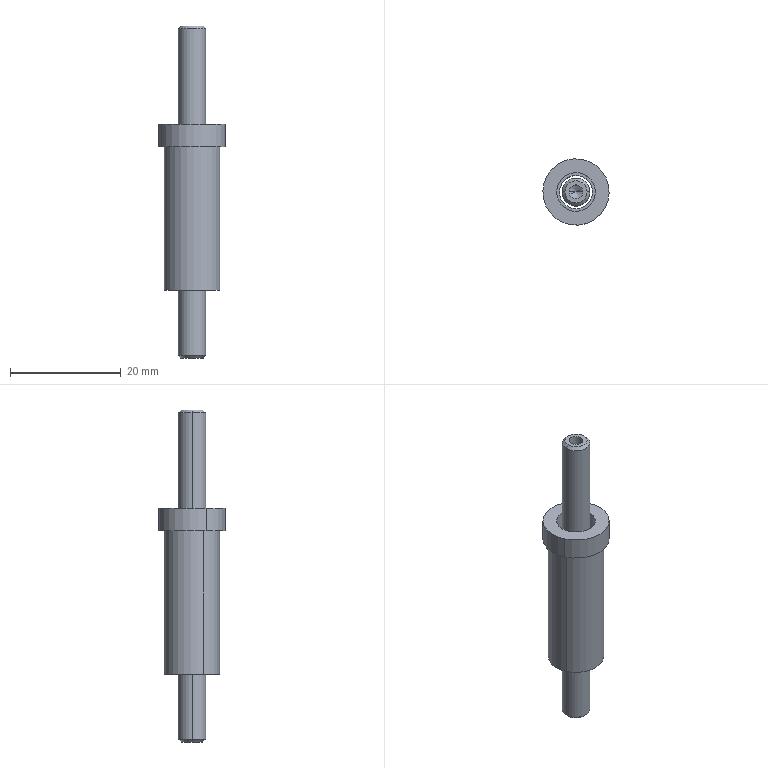Part | NX | features BREP 2 | 2 solids | 31 faces | box 12 x 12 x 60 mm | volume 2642 mm3 | cylinder 16 | cone 8 | plane 7 | commonest cylinder face diameters 2.5 x4 7 x4 5 x2 6 x2 10 x2 12 x2
STEP:
#1=CARTESIAN_POINT('',(-71.096,14.282,-29.5));
#2=VERTEX_POINT('',#1);
#3=CARTESIAN_POINT('',(-70.596,14.282,-30.));
#4=VERTEX_POINT('',#3);
#5=CARTESIAN_POINT('',(-71.096,14.282,-29.5));
#6=DIRECTION('',(-0.7071,0.,0.7071));
#7=VECTOR('',#6,1000.);
#8=LINE('',#5,#7);
#9=EDGE_CURVE('',#2,#4,#8,.F.);
#10=ORIENTED_EDGE('',*,*,#9,.T.);
#11=CARTESIAN_POINT('',(-66.596,14.282,-30.));
#12=VERTEX_POINT('',#11);
#13=CARTESIAN_POINT('',(-68.596,14.282,-30.));
#14=DIRECTION('',(0.,0.,-1.));
#15=DIRECTION('',(1.,0.,0.));
#16=AXIS2_PLACEMENT_3D('',#13,#14,#15);
#17=CIRCLE('',#16,2.);
#18=EDGE_CURVE('',#12,#4,#17,.T.);
#19=ORIENTED_EDGE('',*,*,#18,.F.);
#20=CARTESIAN_POINT('',(-66.096,14.282,-29.5));
#21=VERTEX_POINT('',#20);
#22=CARTESIAN_POINT('',(-66.096,14.282,-29.5));
#23=DIRECTION('',(0.7071,0.,0.7071));
#24=VECTOR('',#23,1000.);
#25=LINE('',#22,#24);
#26=EDGE_CURVE('',#21,#12,#25,.F.);
#27=ORIENTED_EDGE('',*,*,#26,.F.);
#28=CARTESIAN_POINT('',(-68.596,14.282,-29.5));
#29=DIRECTION('',(0.,0.,1.));
#30=DIRECTION('',(1.,0.,0.));
#31=AXIS2_PLACEMENT_3D('',#28,#29,#30);
#32=CIRCLE('',#31,2.5);
#33=EDGE_CURVE('',#2,#21,#32,.T.);
#34=ORIENTED_EDGE('',*,*,#33,.F.);
#35=EDGE_LOOP('',(#10,#19,#27,#34));
#36=FACE_BOUND('',#35,.T.);
#37=CARTESIAN_POINT('',(-68.596,14.282,-29.5));
#38=DIRECTION('',(0.,0.,1.));
#39=DIRECTION('',(1.,0.,0.));
#40=AXIS2_PLACEMENT_3D('',#37,#38,#39);
#41=CONICAL_SURFACE('',#40,2.5,0.7854);
#42=ADVANCED_FACE('',(#36),#41,.T.);
#43=CARTESIAN_POINT('',(-66.596,14.282,30.));
#44=VERTEX_POINT('',#43);
#45=CARTESIAN_POINT('',(-66.096,14.282,29.5));
#46=VERTEX_POINT('',#45);
#47=CARTESIAN_POINT('',(-66.596,14.282,30.));
#48=DIRECTION('',(0.7071,0.,-0.7071));
#49=VECTOR('',#48,1000.);
#50=LINE('',#47,#49);
#51=EDGE_CURVE('',#44,#46,#50,.T.);
#52=ORIENTED_EDGE('',*,*,#51,.F.);
#53=CARTESIAN_POINT('',(-70.596,14.282,30.));
#54=VERTEX_POINT('',#53);
#55=CARTESIAN_POINT('',(-68.596,14.282,30.));
#56=DIRECTION('',(0.,0.,1.));
#57=DIRECTION('',(1.,0.,0.));
#58=AXIS2_PLACEMENT_3D('',#55,#56,#57);
#59=CIRCLE('',#58,2.);
#60=EDGE_CURVE('',#54,#44,#59,.T.);
#61=ORIENTED_EDGE('',*,*,#60,.F.);
#62=CARTESIAN_POINT('',(-71.096,14.282,29.5));
#63=VERTEX_POINT('',#62);
#64=CARTESIAN_POINT('',(-70.596,14.282,30.));
#65=DIRECTION('',(-0.7071,0.,-0.7071));
#66=VECTOR('',#65,1000.);
#67=LINE('',#64,#66);
#68=EDGE_CURVE('',#54,#63,#67,.T.);
#69=ORIENTED_EDGE('',*,*,#68,.T.);
#70=CARTESIAN_POINT('',(-68.596,14.282,29.5));
#71=DIRECTION('',(0.,0.,-1.));
#72=DIRECTION('',(1.,0.,0.));
#73=AXIS2_PLACEMENT_3D('',#70,#71,#72);
#74=CIRCLE('',#73,2.5);
#75=EDGE_CURVE('',#46,#63,#74,.T.);
#76=ORIENTED_EDGE('',*,*,#75,.F.);
#77=EDGE_LOOP('',(#52,#61,#69,#76));
#78=FACE_BOUND('',#77,.T.);
#79=CARTESIAN_POINT('',(-68.596,14.282,30.));
#80=DIRECTION('',(0.,0.,-1.));
#81=DIRECTION('',(-1.,0.,0.));
#82=AXIS2_PLACEMENT_3D('',#79,#80,#81);
#83=CONICAL_SURFACE('',#82,2.,0.7854);
#84=ADVANCED_FACE('',(#78),#83,.T.);
#85=CARTESIAN_POINT('',(-69.846,14.282,30.));
#86=VERTEX_POINT('',#85);
#87=CARTESIAN_POINT('',(-69.846,14.282,22.5));
#88=VERTEX_POINT('',#87);
#89=CARTESIAN_POINT('',(-69.846,14.282,30.));
#90=DIRECTION('',(0.,0.,1.));
#91=VECTOR('',#90,1000.);
#92=LINE('',#89,#91);
#93=EDGE_CURVE('',#86,#88,#92,.F.);
#94=ORIENTED_EDGE('',*,*,#93,.T.);
#95=CARTESIAN_POINT('',(-67.346,14.282,22.5));
#96=VERTEX_POINT('',#95);
#97=CARTESIAN_POINT('',(-68.596,14.282,22.5));
#98=DIRECTION('',(0.,0.,1.));
#99=DIRECTION('',(1.,0.,0.));
#100=AXIS2_PLACEMENT_3D('',#97,#98,#99);
#101=CIRCLE('',#100,1.25);
#102=EDGE_CURVE('',#96,#88,#101,.T.);
#103=ORIENTED_EDGE('',*,*,#102,.F.);
#104=CARTESIAN_POINT('',(-67.346,14.282,30.));
#105=VERTEX_POINT('',#104);
#106=CARTESIAN_POINT('',(-67.346,14.282,30.));
#107=DIRECTION('',(0.,0.,1.));
#108=VECTOR('',#107,1000.);
#109=LINE('',#106,#108);
#110=EDGE_CURVE('',#105,#96,#109,.F.);
#111=ORIENTED_EDGE('',*,*,#110,.F.);
#112=CARTESIAN_POINT('',(-68.596,14.282,30.));
#113=DIRECTION('',(0.,0.,1.));
#114=DIRECTION('',(1.,0.,0.));
#115=AXIS2_PLACEMENT_3D('',#112,#113,#114);
#116=CIRCLE('',#115,1.25);
#117=EDGE_CURVE('',#105,#86,#116,.T.);
#118=ORIENTED_EDGE('',*,*,#117,.T.);
#119=EDGE_LOOP('',(#94,#103,#111,#118));
#120=FACE_BOUND('',#119,.T.);
#121=CARTESIAN_POINT('',(-68.596,14.282,30.));
#122=DIRECTION('',(0.,0.,1.));
#123=DIRECTION('',(1.,0.,0.));
#124=AXIS2_PLACEMENT_3D('',#121,#122,#123);
#125=CYLINDRICAL_SURFACE('',#124,1.25);
#126=ADVANCED_FACE('',(#120),#125,.F.);
#127=CARTESIAN_POINT('',(-68.596,14.282,21.749));
#128=VERTEX_POINT('',#127);
#129=CARTESIAN_POINT('',(-69.846,14.282,22.5));
#130=DIRECTION('',(-0.8572,0.,0.515));
#131=VECTOR('',#130,1000.);
#132=LINE('',#129,#131);
#133=EDGE_CURVE('',#128,#88,#132,.T.);
#134=ORIENTED_EDGE('',*,*,#133,.F.);
#135=CARTESIAN_POINT('',(-67.346,14.282,22.5));
#136=DIRECTION('',(0.8572,0.,0.515));
#137=VECTOR('',#136,1000.);
#138=LINE('',#135,#137);
#139=EDGE_CURVE('',#128,#96,#138,.T.);
#140=ORIENTED_EDGE('',*,*,#139,.T.);
#141=ORIENTED_EDGE('',*,*,#102,.T.);
#142=EDGE_LOOP('',(#134,#140,#141));
#143=FACE_BOUND('',#142,.T.);
#144=CARTESIAN_POINT('',(-68.596,14.282,22.5));
#145=DIRECTION('',(0.,0.,1.));
#146=DIRECTION('',(1.,0.,0.));
#147=AXIS2_PLACEMENT_3D('',#144,#145,#146);
#148=CONICAL_SURFACE('',#147,1.25,1.03);
#149=ADVANCED_FACE('',(#143),#148,.F.);
#150=CARTESIAN_POINT('',(-67.346,14.282,-22.5));
#151=VERTEX_POINT('',#150);
#152=CARTESIAN_POINT('',(-67.346,14.282,-30.));
#153=VERTEX_POINT('',#152);
#154=CARTESIAN_POINT('',(-67.346,14.282,-30.));
#155=DIRECTION('',(0.,0.,-1.));
#156=VECTOR('',#155,1000.);
#157=LINE('',#154,#156);
#158=EDGE_CURVE('',#151,#153,#157,.T.);
#159=ORIENTED_EDGE('',*,*,#158,.F.);
#160=CARTESIAN_POINT('',(-69.846,14.282,-22.5));
#161=VERTEX_POINT('',#160);
#162=CARTESIAN_POINT('',(-68.596,14.282,-22.5));
#163=DIRECTION('',(0.,0.,-1.));
#164=DIRECTION('',(-1.,0.,0.));
#165=AXIS2_PLACEMENT_3D('',#162,#163,#164);
#166=CIRCLE('',#165,1.25);
#167=EDGE_CURVE('',#161,#151,#166,.T.);
#168=ORIENTED_EDGE('',*,*,#167,.F.);
#169=CARTESIAN_POINT('',(-69.846,14.282,-30.));
#170=VERTEX_POINT('',#169);
#171=CARTESIAN_POINT('',(-69.846,14.282,-30.));
#172=DIRECTION('',(0.,0.,-1.));
#173=VECTOR('',#172,1000.);
#174=LINE('',#171,#173);
#175=EDGE_CURVE('',#161,#170,#174,.T.);
#176=ORIENTED_EDGE('',*,*,#175,.T.);
#177=CARTESIAN_POINT('',(-68.596,14.282,-30.));
#178=DIRECTION('',(0.,0.,-1.));
#179=DIRECTION('',(-1.,0.,0.));
#180=AXIS2_PLACEMENT_3D('',#177,#178,#179);
#181=CIRCLE('',#180,1.25);
#182=EDGE_CURVE('',#170,#153,#181,.T.);
#183=ORIENTED_EDGE('',*,*,#182,.T.);
#184=EDGE_LOOP('',(#159,#168,#176,#183));
#185=FACE_BOUND('',#184,.T.);
#186=CARTESIAN_POINT('',(-68.596,14.282,-30.));
#187=DIRECTION('',(0.,0.,-1.));
#188=DIRECTION('',(-1.,0.,0.));
#189=AXIS2_PLACEMENT_3D('',#186,#187,#188);
#190=CYLINDRICAL_SURFACE('',#189,1.25);
#191=ADVANCED_FACE('',(#185),#190,.F.);
#192=CARTESIAN_POINT('',(-68.596,14.282,-21.749));
#193=VERTEX_POINT('',#192);
#194=CARTESIAN_POINT('',(-67.346,14.282,-22.5));
#195=DIRECTION('',(0.8572,0.,-0.515));
#196=VECTOR('',#195,1000.);
#197=LINE('',#194,#196);
#198=EDGE_CURVE('',#151,#193,#197,.F.);
#199=ORIENTED_EDGE('',*,*,#198,.T.);
#200=CARTESIAN_POINT('',(-69.846,14.282,-22.5));
#201=DIRECTION('',(-0.8572,0.,-0.515));
#202=VECTOR('',#201,1000.);
#203=LINE('',#200,#202);
#204=EDGE_CURVE('',#161,#193,#203,.F.);
#205=ORIENTED_EDGE('',*,*,#204,.F.);
#206=ORIENTED_EDGE('',*,*,#167,.T.);
#207=EDGE_LOOP('',(#199,#205,#206));
#208=FACE_BOUND('',#207,.T.);
#209=CARTESIAN_POINT('',(-68.596,14.282,-22.5));
#210=DIRECTION('',(0.,0.,-1.));
#211=DIRECTION('',(-1.,0.,0.));
#212=AXIS2_PLACEMENT_3D('',#209,#210,#211);
#213=CONICAL_SURFACE('',#212,1.25,1.03);
#214=ADVANCED_FACE('',(#208),#213,.F.);
#215=ORIENTED_EDGE('',*,*,#182,.F.);
#216=CARTESIAN_POINT('',(-68.596,14.282,-30.));
#217=DIRECTION('',(0.,0.,-1.));
#218=DIRECTION('',(-1.,0.,0.));
#219=AXIS2_PLACEMENT_3D('',#216,#217,#218);
#220=CIRCLE('',#219,1.25);
#221=EDGE_CURVE('',#153,#170,#220,.T.);
#222=ORIENTED_EDGE('',*,*,#221,.F.);
#223=EDGE_LOOP('',(#215,#222));
#224=FACE_BOUND('',#223,.T.);
#225=ORIENTED_EDGE('',*,*,#18,.T.);
#226=CARTESIAN_POINT('',(-68.596,14.282,-30.));
#227=DIRECTION('',(0.,0.,-1.));
#228=DIRECTION('',(1.,0.,0.));
#229=AXIS2_PLACEMENT_3D('',#226,#227,#228);
#230=CIRCLE('',#229,2.);
#231=EDGE_CURVE('',#4,#12,#230,.T.);
#232=ORIENTED_EDGE('',*,*,#231,.T.);
#233=EDGE_LOOP('',(#225,#232));
#234=FACE_BOUND('',#233,.T.);
#235=CARTESIAN_POINT('',(-68.596,14.282,-30.));
#236=DIRECTION('',(0.,0.,1.));
#237=DIRECTION('',(1.,0.,0.));
#238=AXIS2_PLACEMENT_3D('',#235,#236,#237);
#239=PLANE('',#238);
#240=ADVANCED_FACE('',(#224,#234),#239,.F.);
#241=ORIENTED_EDGE('',*,*,#117,.F.);
#242=CARTESIAN_POINT('',(-68.596,14.282,30.));
#243=DIRECTION('',(0.,0.,1.));
#244=DIRECTION('',(1.,0.,0.));
#245=AXIS2_PLACEMENT_3D('',#242,#243,#244);
#246=CIRCLE('',#245,1.25);
#247=EDGE_CURVE('',#86,#105,#246,.T.);
#248=ORIENTED_EDGE('',*,*,#247,.F.);
#249=EDGE_LOOP('',(#241,#248));
#250=FACE_BOUND('',#249,.T.);
#251=ORIENTED_EDGE('',*,*,#60,.T.);
#252=CARTESIAN_POINT('',(-68.596,14.282,30.));
#253=DIRECTION('',(0.,0.,1.));
#254=DIRECTION('',(1.,0.,0.));
#255=AXIS2_PLACEMENT_3D('',#252,#253,#254);
#256=CIRCLE('',#255,2.);
#257=EDGE_CURVE('',#44,#54,#256,.T.);
#258=ORIENTED_EDGE('',*,*,#257,.T.);
#259=EDGE_LOOP('',(#251,#258));
#260=FACE_BOUND('',#259,.T.);
#261=CARTESIAN_POINT('',(-68.596,14.282,30.));
#262=DIRECTION('',(0.,0.,1.));
#263=DIRECTION('',(1.,0.,0.));
#264=AXIS2_PLACEMENT_3D('',#261,#262,#263);
#265=PLANE('',#264);
#266=ADVANCED_FACE('',(#250,#260),#265,.T.);
#267=CARTESIAN_POINT('',(-66.096,14.282,30.));
#268=DIRECTION('',(0.,0.,-1.));
#269=VECTOR('',#268,1000.);
#270=LINE('',#267,#269);
#271=EDGE_CURVE('',#46,#21,#270,.T.);
#272=ORIENTED_EDGE('',*,*,#271,.F.);
#273=ORIENTED_EDGE('',*,*,#75,.T.);
#274=CARTESIAN_POINT('',(-71.096,14.282,30.));
#275=DIRECTION('',(0.,0.,-1.));
#276=VECTOR('',#275,1000.);
#277=LINE('',#274,#276);
#278=EDGE_CURVE('',#63,#2,#277,.T.);
#279=ORIENTED_EDGE('',*,*,#278,.T.);
#280=ORIENTED_EDGE('',*,*,#33,.T.);
#281=EDGE_LOOP('',(#272,#273,#279,#280));
#282=FACE_BOUND('',#281,.T.);
#283=CARTESIAN_POINT('',(-68.596,14.282,30.));
#284=DIRECTION('',(0.,0.,-1.));
#285=DIRECTION('',(-1.,0.,0.));
#286=AXIS2_PLACEMENT_3D('',#283,#284,#285);
#287=CYLINDRICAL_SURFACE('',#286,2.5);
#288=ADVANCED_FACE('',(#282),#287,.T.);
#289=CARTESIAN_POINT('',(-68.596,14.282,29.5));
#290=DIRECTION('',(0.,0.,-1.));
#291=DIRECTION('',(1.,0.,0.));
#292=AXIS2_PLACEMENT_3D('',#289,#290,#291);
#293=CIRCLE('',#292,2.5);
#294=EDGE_CURVE('',#63,#46,#293,.T.);
#295=ORIENTED_EDGE('',*,*,#294,.T.);
#296=ORIENTED_EDGE('',*,*,#271,.T.);
#297=CARTESIAN_POINT('',(-68.596,14.282,-29.5));
#298=DIRECTION('',(0.,0.,1.));
#299=DIRECTION('',(1.,0.,0.));
#300=AXIS2_PLACEMENT_3D('',#297,#298,#299);
#301=CIRCLE('',#300,2.5);
#302=EDGE_CURVE('',#21,#2,#301,.T.);
#303=ORIENTED_EDGE('',*,*,#302,.T.);
#304=ORIENTED_EDGE('',*,*,#278,.F.);
#305=EDGE_LOOP('',(#295,#296,#303,#304));
#306=FACE_BOUND('',#305,.T.);
#307=CARTESIAN_POINT('',(-68.596,14.282,30.));
#308=DIRECTION('',(0.,0.,-1.));
#309=DIRECTION('',(-1.,0.,0.));
#310=AXIS2_PLACEMENT_3D('',#307,#308,#309);
#311=CYLINDRICAL_SURFACE('',#310,2.5);
#312=ADVANCED_FACE('',(#306),#311,.T.);
#313=ORIENTED_EDGE('',*,*,#204,.T.);
#314=ORIENTED_EDGE('',*,*,#198,.F.);
#315=CARTESIAN_POINT('',(-68.596,14.282,-22.5));
#316=DIRECTION('',(0.,0.,-1.));
#317=DIRECTION('',(-1.,0.,0.));
#318=AXIS2_PLACEMENT_3D('',#315,#316,#317);
#319=CIRCLE('',#318,1.25);
#320=EDGE_CURVE('',#151,#161,#319,.T.);
#321=ORIENTED_EDGE('',*,*,#320,.T.);
#322=EDGE_LOOP('',(#313,#314,#321));
#323=FACE_BOUND('',#322,.T.);
#324=CARTESIAN_POINT('',(-68.596,14.282,-22.5));
#325=DIRECTION('',(0.,0.,-1.));
#326=DIRECTION('',(-1.,0.,0.));
#327=AXIS2_PLACEMENT_3D('',#324,#325,#326);
#328=CONICAL_SURFACE('',#327,1.25,1.03);
#329=ADVANCED_FACE('',(#323),#328,.F.);
#330=ORIENTED_EDGE('',*,*,#320,.F.);
#331=ORIENTED_EDGE('',*,*,#158,.T.);
#332=ORIENTED_EDGE('',*,*,#221,.T.);
#333=ORIENTED_EDGE('',*,*,#175,.F.);
#334=EDGE_LOOP('',(#330,#331,#332,#333));
#335=FACE_BOUND('',#334,.T.);
#336=CARTESIAN_POINT('',(-68.596,14.282,-30.));
#337=DIRECTION('',(0.,0.,-1.));
#338=DIRECTION('',(-1.,0.,0.));
#339=AXIS2_PLACEMENT_3D('',#336,#337,#338);
#340=CYLINDRICAL_SURFACE('',#339,1.25);
#341=ADVANCED_FACE('',(#335),#340,.F.);
#342=ORIENTED_EDGE('',*,*,#139,.F.);
#343=ORIENTED_EDGE('',*,*,#133,.T.);
#344=CARTESIAN_POINT('',(-68.596,14.282,22.5));
#345=DIRECTION('',(0.,0.,1.));
#346=DIRECTION('',(1.,0.,0.));
#347=AXIS2_PLACEMENT_3D('',#344,#345,#346);
#348=CIRCLE('',#347,1.25);
#349=EDGE_CURVE('',#88,#96,#348,.T.);
#350=ORIENTED_EDGE('',*,*,#349,.T.);
#351=EDGE_LOOP('',(#342,#343,#350));
#352=FACE_BOUND('',#351,.T.);
#353=CARTESIAN_POINT('',(-68.596,14.282,22.5));
#354=DIRECTION('',(0.,0.,1.));
#355=DIRECTION('',(1.,0.,0.));
#356=AXIS2_PLACEMENT_3D('',#353,#354,#355);
#357=CONICAL_SURFACE('',#356,1.25,1.03);
#358=ADVANCED_FACE('',(#352),#357,.F.);
#359=ORIENTED_EDGE('',*,*,#349,.F.);
#360=ORIENTED_EDGE('',*,*,#93,.F.);
#361=ORIENTED_EDGE('',*,*,#247,.T.);
#362=ORIENTED_EDGE('',*,*,#110,.T.);
#363=EDGE_LOOP('',(#359,#360,#361,#362));
#364=FACE_BOUND('',#363,.T.);
#365=CARTESIAN_POINT('',(-68.596,14.282,30.));
#366=DIRECTION('',(0.,0.,1.));
#367=DIRECTION('',(1.,0.,0.));
#368=AXIS2_PLACEMENT_3D('',#365,#366,#367);
#369=CYLINDRICAL_SURFACE('',#368,1.25);
#370=ADVANCED_FACE('',(#364),#369,.F.);
#371=ORIENTED_EDGE('',*,*,#257,.F.);
#372=ORIENTED_EDGE('',*,*,#51,.T.);
#373=ORIENTED_EDGE('',*,*,#294,.F.);
#374=ORIENTED_EDGE('',*,*,#68,.F.);
#375=EDGE_LOOP('',(#371,#372,#373,#374));
#376=FACE_BOUND('',#375,.T.);
#377=CARTESIAN_POINT('',(-68.596,14.282,30.));
#378=DIRECTION('',(0.,0.,-1.));
#379=DIRECTION('',(-1.,0.,0.));
#380=AXIS2_PLACEMENT_3D('',#377,#378,#379);
#381=CONICAL_SURFACE('',#380,2.,0.7854);
#382=ADVANCED_FACE('',(#376),#381,.T.);
#383=ORIENTED_EDGE('',*,*,#231,.F.);
#384=ORIENTED_EDGE('',*,*,#9,.F.);
#385=ORIENTED_EDGE('',*,*,#302,.F.);
#386=ORIENTED_EDGE('',*,*,#26,.T.);
#387=EDGE_LOOP('',(#383,#384,#385,#386));
#388=FACE_BOUND('',#387,.T.);
#389=CARTESIAN_POINT('',(-68.596,14.282,-29.5));
#390=DIRECTION('',(0.,0.,1.));
#391=DIRECTION('',(1.,0.,0.));
#392=AXIS2_PLACEMENT_3D('',#389,#390,#391);
#393=CONICAL_SURFACE('',#392,2.5,0.7854);
#394=ADVANCED_FACE('',(#388),#393,.T.);
#395=CLOSED_SHELL('',(#42,#84,#126,#149,#191,#214,#240,#266,#288,#312,#329,#341,#358,#370,#382,#394));
#396=MANIFOLD_SOLID_BREP('',#395);
#397=CARTESIAN_POINT('',(-71.767,12.8,-12.8));
#398=VERTEX_POINT('',#397);
#399=CARTESIAN_POINT('',(-65.425,15.764,-12.8));
#400=VERTEX_POINT('',#399);
#401=CARTESIAN_POINT('',(-68.596,14.282,-12.8));
#402=DIRECTION('',(0.,0.,-1.));
#403=DIRECTION('',(-0.9059,-0.4234,0.));
#404=AXIS2_PLACEMENT_3D('',#401,#402,#403);
#405=CIRCLE('',#404,3.5);
#406=EDGE_CURVE('',#398,#400,#405,.T.);
#407=ORIENTED_EDGE('',*,*,#406,.T.);
#408=CARTESIAN_POINT('',(-68.596,14.282,-12.8));
#409=DIRECTION('',(0.,0.,-1.));
#410=DIRECTION('',(-0.9059,-0.4234,0.));
#411=AXIS2_PLACEMENT_3D('',#408,#409,#410);
#412=CIRCLE('',#411,3.5);
#413=EDGE_CURVE('',#400,#398,#412,.T.);
#414=ORIENTED_EDGE('',*,*,#413,.T.);
#415=EDGE_LOOP('',(#407,#414));
#416=FACE_BOUND('',#415,.T.);
#417=CARTESIAN_POINT('',(-65.878,15.552,-12.8));
#418=VERTEX_POINT('',#417);
#419=CARTESIAN_POINT('',(-71.314,13.012,-12.8));
#420=VERTEX_POINT('',#419);
#421=CARTESIAN_POINT('',(-68.596,14.282,-12.8));
#422=DIRECTION('',(0.,0.,-1.));
#423=DIRECTION('',(-0.9059,-0.4234,0.));
#424=AXIS2_PLACEMENT_3D('',#421,#422,#423);
#425=CIRCLE('',#424,3.);
#426=EDGE_CURVE('',#418,#420,#425,.T.);
#427=ORIENTED_EDGE('',*,*,#426,.F.);
#428=CARTESIAN_POINT('',(-68.596,14.282,-12.8));
#429=DIRECTION('',(0.,0.,-1.));
#430=DIRECTION('',(-0.9059,-0.4234,0.));
#431=AXIS2_PLACEMENT_3D('',#428,#429,#430);
#432=CIRCLE('',#431,3.);
#433=EDGE_CURVE('',#420,#418,#432,.T.);
#434=ORIENTED_EDGE('',*,*,#433,.F.);
#435=EDGE_LOOP('',(#427,#434));
#436=FACE_BOUND('',#435,.T.);
#437=CARTESIAN_POINT('',(-68.596,14.282,-12.8));
#438=DIRECTION('',(0.,0.,-1.));
#439=DIRECTION('',(-0.9059,-0.4234,0.));
#440=AXIS2_PLACEMENT_3D('',#437,#438,#439);
#441=PLANE('',#440);
#442=ADVANCED_FACE('',(#416,#436),#441,.T.);
#443=CARTESIAN_POINT('',(-65.425,15.764,-17.8));
#444=VERTEX_POINT('',#443);
#445=CARTESIAN_POINT('',(-65.425,15.764,-12.8));
#446=DIRECTION('',(0.,0.,-1.));
#447=VECTOR('',#446,1000.);
#448=LINE('',#445,#447);
#449=EDGE_CURVE('',#400,#444,#448,.T.);
#450=ORIENTED_EDGE('',*,*,#449,.F.);
#451=ORIENTED_EDGE('',*,*,#406,.F.);
#452=CARTESIAN_POINT('',(-71.767,12.8,-17.8));
#453=VERTEX_POINT('',#452);
#454=CARTESIAN_POINT('',(-71.767,12.8,-12.8));
#455=DIRECTION('',(0.,0.,-1.));
#456=VECTOR('',#455,1000.);
#457=LINE('',#454,#456);
#458=EDGE_CURVE('',#398,#453,#457,.T.);
#459=ORIENTED_EDGE('',*,*,#458,.T.);
#460=CARTESIAN_POINT('',(-68.596,14.282,-17.8));
#461=DIRECTION('',(0.,0.,-1.));
#462=DIRECTION('',(-0.9059,-0.4234,0.));
#463=AXIS2_PLACEMENT_3D('',#460,#461,#462);
#464=CIRCLE('',#463,3.5);
#465=EDGE_CURVE('',#453,#444,#464,.T.);
#466=ORIENTED_EDGE('',*,*,#465,.T.);
#467=EDGE_LOOP('',(#450,#451,#459,#466));
#468=FACE_BOUND('',#467,.T.);
#469=CARTESIAN_POINT('',(-68.596,14.282,-12.8));
#470=DIRECTION('',(0.,0.,-1.));
#471=DIRECTION('',(-0.9059,-0.4234,0.));
#472=AXIS2_PLACEMENT_3D('',#469,#470,#471);
#473=CYLINDRICAL_SURFACE('',#472,3.5);
#474=ADVANCED_FACE('',(#468),#473,.F.);
#475=CARTESIAN_POINT('',(-65.425,15.764,7.2));
#476=VERTEX_POINT('',#475);
#477=CARTESIAN_POINT('',(-71.767,12.8,7.2));
#478=VERTEX_POINT('',#477);
#479=CARTESIAN_POINT('',(-68.596,14.282,7.2));
#480=DIRECTION('',(0.,0.,1.));
#481=DIRECTION('',(0.9059,0.4234,0.));
#482=AXIS2_PLACEMENT_3D('',#479,#480,#481);
#483=CIRCLE('',#482,3.5);
#484=EDGE_CURVE('',#476,#478,#483,.T.);
#485=ORIENTED_EDGE('',*,*,#484,.T.);
#486=CARTESIAN_POINT('',(-68.596,14.282,7.2));
#487=DIRECTION('',(0.,0.,1.));
#488=DIRECTION('',(0.9059,0.4234,0.));
#489=AXIS2_PLACEMENT_3D('',#486,#487,#488);
#490=CIRCLE('',#489,3.5);
#491=EDGE_CURVE('',#478,#476,#490,.T.);
#492=ORIENTED_EDGE('',*,*,#491,.T.);
#493=EDGE_LOOP('',(#485,#492));
#494=FACE_BOUND('',#493,.T.);
#495=CARTESIAN_POINT('',(-65.878,15.552,7.2));
#496=VERTEX_POINT('',#495);
#497=CARTESIAN_POINT('',(-71.314,13.012,7.2));
#498=VERTEX_POINT('',#497);
#499=CARTESIAN_POINT('',(-68.596,14.282,7.2));
#500=DIRECTION('',(0.,0.,1.));
#501=DIRECTION('',(0.9059,0.4234,0.));
#502=AXIS2_PLACEMENT_3D('',#499,#500,#501);
#503=CIRCLE('',#502,3.);
#504=EDGE_CURVE('',#496,#498,#503,.T.);
#505=ORIENTED_EDGE('',*,*,#504,.F.);
#506=CARTESIAN_POINT('',(-68.596,14.282,7.2));
#507=DIRECTION('',(0.,0.,1.));
#508=DIRECTION('',(0.9059,0.4234,0.));
#509=AXIS2_PLACEMENT_3D('',#506,#507,#508);
#510=CIRCLE('',#509,3.);
#511=EDGE_CURVE('',#498,#496,#510,.T.);
#512=ORIENTED_EDGE('',*,*,#511,.F.);
#513=EDGE_LOOP('',(#505,#512));
#514=FACE_BOUND('',#513,.T.);
#515=CARTESIAN_POINT('',(-68.596,14.282,7.2));
#516=DIRECTION('',(0.,0.,1.));
#517=DIRECTION('',(0.9059,0.4234,0.));
#518=AXIS2_PLACEMENT_3D('',#515,#516,#517);
#519=PLANE('',#518);
#520=ADVANCED_FACE('',(#494,#514),#519,.T.);
#521=CARTESIAN_POINT('',(-71.767,12.8,12.2));
#522=VERTEX_POINT('',#521);
#523=CARTESIAN_POINT('',(-71.767,12.8,7.2));
#524=DIRECTION('',(0.,0.,1.));
#525=VECTOR('',#524,1000.);
#526=LINE('',#523,#525);
#527=EDGE_CURVE('',#522,#478,#526,.F.);
#528=ORIENTED_EDGE('',*,*,#527,.T.);
#529=ORIENTED_EDGE('',*,*,#484,.F.);
#530=CARTESIAN_POINT('',(-65.425,15.764,12.2));
#531=VERTEX_POINT('',#530);
#532=CARTESIAN_POINT('',(-65.425,15.764,7.2));
#533=DIRECTION('',(0.,0.,1.));
#534=VECTOR('',#533,1000.);
#535=LINE('',#532,#534);
#536=EDGE_CURVE('',#531,#476,#535,.F.);
#537=ORIENTED_EDGE('',*,*,#536,.F.);
#538=CARTESIAN_POINT('',(-68.596,14.282,12.2));
#539=DIRECTION('',(0.,0.,1.));
#540=DIRECTION('',(0.9059,0.4234,0.));
#541=AXIS2_PLACEMENT_3D('',#538,#539,#540);
#542=CIRCLE('',#541,3.5);
#543=EDGE_CURVE('',#531,#522,#542,.T.);
#544=ORIENTED_EDGE('',*,*,#543,.T.);
#545=EDGE_LOOP('',(#528,#529,#537,#544));
#546=FACE_BOUND('',#545,.T.);
#547=CARTESIAN_POINT('',(-68.596,14.282,7.2));
#548=DIRECTION('',(0.,0.,1.));
#549=DIRECTION('',(0.9059,0.4234,0.));
#550=AXIS2_PLACEMENT_3D('',#547,#548,#549);
#551=CYLINDRICAL_SURFACE('',#550,3.5);
#552=ADVANCED_FACE('',(#546),#551,.F.);
#553=CARTESIAN_POINT('',(-63.161,16.822,8.2));
#554=VERTEX_POINT('',#553);
#555=CARTESIAN_POINT('',(-74.032,11.741,8.2));
#556=VERTEX_POINT('',#555);
#557=CARTESIAN_POINT('',(-68.596,14.282,8.2));
#558=DIRECTION('',(0.,0.,1.));
#559=DIRECTION('',(0.9059,0.4234,0.));
#560=AXIS2_PLACEMENT_3D('',#557,#558,#559);
#561=CIRCLE('',#560,6.);
#562=EDGE_CURVE('',#554,#556,#561,.T.);
#563=ORIENTED_EDGE('',*,*,#562,.F.);
#564=CARTESIAN_POINT('',(-68.596,14.282,8.2));
#565=DIRECTION('',(0.,0.,1.));
#566=DIRECTION('',(0.9059,0.4234,0.));
#567=AXIS2_PLACEMENT_3D('',#564,#565,#566);
#568=CIRCLE('',#567,6.);
#569=EDGE_CURVE('',#556,#554,#568,.T.);
#570=ORIENTED_EDGE('',*,*,#569,.F.);
#571=EDGE_LOOP('',(#563,#570));
#572=FACE_BOUND('',#571,.T.);
#573=CARTESIAN_POINT('',(-64.067,16.399,8.2));
#574=VERTEX_POINT('',#573);
#575=CARTESIAN_POINT('',(-73.126,12.165,8.2));
#576=VERTEX_POINT('',#575);
#577=CARTESIAN_POINT('',(-68.596,14.282,8.2));
#578=DIRECTION('',(0.,0.,1.));
#579=DIRECTION('',(0.9059,0.4234,0.));
#580=AXIS2_PLACEMENT_3D('',#577,#578,#579);
#581=CIRCLE('',#580,5.);
#582=EDGE_CURVE('',#574,#576,#581,.T.);
#583=ORIENTED_EDGE('',*,*,#582,.T.);
#584=CARTESIAN_POINT('',(-68.596,14.282,8.2));
#585=DIRECTION('',(0.,0.,1.));
#586=DIRECTION('',(0.9059,0.4234,0.));
#587=AXIS2_PLACEMENT_3D('',#584,#585,#586);
#588=CIRCLE('',#587,5.);
#589=EDGE_CURVE('',#576,#574,#588,.T.);
#590=ORIENTED_EDGE('',*,*,#589,.T.);
#591=EDGE_LOOP('',(#583,#590));
#592=FACE_BOUND('',#591,.T.);
#593=CARTESIAN_POINT('',(-68.596,14.282,8.2));
#594=DIRECTION('',(0.,0.,1.));
#595=DIRECTION('',(0.9059,0.4234,0.));
#596=AXIS2_PLACEMENT_3D('',#593,#594,#595);
#597=PLANE('',#596);
#598=ADVANCED_FACE('',(#572,#592),#597,.F.);
#599=CARTESIAN_POINT('',(-74.032,11.741,12.2));
#600=VERTEX_POINT('',#599);
#601=CARTESIAN_POINT('',(-74.032,11.741,8.2));
#602=DIRECTION('',(0.,0.,1.));
#603=VECTOR('',#602,1000.);
#604=LINE('',#601,#603);
#605=EDGE_CURVE('',#600,#556,#604,.F.);
#606=ORIENTED_EDGE('',*,*,#605,.T.);
#607=ORIENTED_EDGE('',*,*,#569,.T.);
#608=CARTESIAN_POINT('',(-63.161,16.822,12.2));
#609=VERTEX_POINT('',#608);
#610=CARTESIAN_POINT('',(-63.161,16.822,8.2));
#611=DIRECTION('',(0.,0.,1.));
#612=VECTOR('',#611,1000.);
#613=LINE('',#610,#612);
#614=EDGE_CURVE('',#609,#554,#613,.F.);
#615=ORIENTED_EDGE('',*,*,#614,.F.);
#616=CARTESIAN_POINT('',(-68.596,14.282,12.2));
#617=DIRECTION('',(0.,0.,1.));
#618=DIRECTION('',(0.9059,0.4234,0.));
#619=AXIS2_PLACEMENT_3D('',#616,#617,#618);
#620=CIRCLE('',#619,6.);
#621=EDGE_CURVE('',#600,#609,#620,.T.);
#622=ORIENTED_EDGE('',*,*,#621,.F.);
#623=EDGE_LOOP('',(#606,#607,#615,#622));
#624=FACE_BOUND('',#623,.T.);
#625=CARTESIAN_POINT('',(-68.596,14.282,8.2));
#626=DIRECTION('',(0.,0.,1.));
#627=DIRECTION('',(0.9059,0.4234,0.));
#628=AXIS2_PLACEMENT_3D('',#625,#626,#627);
#629=CYLINDRICAL_SURFACE('',#628,6.);
#630=ADVANCED_FACE('',(#624),#629,.T.);
#631=CARTESIAN_POINT('',(-68.596,14.282,12.2));
#632=DIRECTION('',(0.,0.,1.));
#633=DIRECTION('',(0.9059,0.4234,0.));
#634=AXIS2_PLACEMENT_3D('',#631,#632,#633);
#635=CIRCLE('',#634,6.);
#636=EDGE_CURVE('',#609,#600,#635,.T.);
#637=ORIENTED_EDGE('',*,*,#636,.T.);
#638=ORIENTED_EDGE('',*,*,#621,.T.);
#639=EDGE_LOOP('',(#637,#638));
#640=FACE_BOUND('',#639,.T.);
#641=ORIENTED_EDGE('',*,*,#543,.F.);
#642=CARTESIAN_POINT('',(-68.596,14.282,12.2));
#643=DIRECTION('',(0.,0.,1.));
#644=DIRECTION('',(0.9059,0.4234,0.));
#645=AXIS2_PLACEMENT_3D('',#642,#643,#644);
#646=CIRCLE('',#645,3.5);
#647=EDGE_CURVE('',#522,#531,#646,.T.);
#648=ORIENTED_EDGE('',*,*,#647,.F.);
#649=EDGE_LOOP('',(#641,#648));
#650=FACE_BOUND('',#649,.T.);
#651=CARTESIAN_POINT('',(-68.596,14.282,12.2));
#652=DIRECTION('',(0.,0.,-1.));
#653=DIRECTION('',(-0.9059,-0.4234,0.));
#654=AXIS2_PLACEMENT_3D('',#651,#652,#653);
#655=PLANE('',#654);
#656=ADVANCED_FACE('',(#640,#650),#655,.F.);
#657=CARTESIAN_POINT('',(-64.067,16.399,-17.8));
#658=VERTEX_POINT('',#657);
#659=CARTESIAN_POINT('',(-73.126,12.165,-17.8));
#660=VERTEX_POINT('',#659);
#661=CARTESIAN_POINT('',(-68.596,14.282,-17.8));
#662=DIRECTION('',(0.,0.,-1.));
#663=DIRECTION('',(-0.9059,-0.4234,0.));
#664=AXIS2_PLACEMENT_3D('',#661,#662,#663);
#665=CIRCLE('',#664,5.);
#666=EDGE_CURVE('',#658,#660,#665,.T.);
#667=ORIENTED_EDGE('',*,*,#666,.T.);
#668=CARTESIAN_POINT('',(-68.596,14.282,-17.8));
#669=DIRECTION('',(0.,0.,-1.));
#670=DIRECTION('',(-0.9059,-0.4234,0.));
#671=AXIS2_PLACEMENT_3D('',#668,#669,#670);
#672=CIRCLE('',#671,5.);
#673=EDGE_CURVE('',#660,#658,#672,.T.);
#674=ORIENTED_EDGE('',*,*,#673,.T.);
#675=EDGE_LOOP('',(#667,#674));
#676=FACE_BOUND('',#675,.T.);
#677=ORIENTED_EDGE('',*,*,#465,.F.);
#678=CARTESIAN_POINT('',(-68.596,14.282,-17.8));
#679=DIRECTION('',(0.,0.,-1.));
#680=DIRECTION('',(-0.9059,-0.4234,0.));
#681=AXIS2_PLACEMENT_3D('',#678,#679,#680);
#682=CIRCLE('',#681,3.5);
#683=EDGE_CURVE('',#444,#453,#682,.T.);
#684=ORIENTED_EDGE('',*,*,#683,.F.);
#685=EDGE_LOOP('',(#677,#684));
#686=FACE_BOUND('',#685,.T.);
#687=CARTESIAN_POINT('',(-68.596,14.282,-17.8));
#688=DIRECTION('',(0.,0.,-1.));
#689=DIRECTION('',(-0.9059,-0.4234,0.));
#690=AXIS2_PLACEMENT_3D('',#687,#688,#689);
#691=PLANE('',#690);
#692=ADVANCED_FACE('',(#676,#686),#691,.T.);
#693=CARTESIAN_POINT('',(-73.126,12.165,-17.8));
#694=DIRECTION('',(0.,0.,1.));
#695=VECTOR('',#694,1000.);
#696=LINE('',#693,#695);
#697=EDGE_CURVE('',#576,#660,#696,.F.);
#698=ORIENTED_EDGE('',*,*,#697,.T.);
#699=ORIENTED_EDGE('',*,*,#666,.F.);
#700=CARTESIAN_POINT('',(-64.067,16.399,-17.8));
#701=DIRECTION('',(0.,0.,1.));
#702=VECTOR('',#701,1000.);
#703=LINE('',#700,#702);
#704=EDGE_CURVE('',#574,#658,#703,.F.);
#705=ORIENTED_EDGE('',*,*,#704,.F.);
#706=ORIENTED_EDGE('',*,*,#589,.F.);
#707=EDGE_LOOP('',(#698,#699,#705,#706));
#708=FACE_BOUND('',#707,.T.);
#709=CARTESIAN_POINT('',(-68.596,14.282,-17.8));
#710=DIRECTION('',(0.,0.,1.));
#711=DIRECTION('',(0.9059,0.4234,0.));
#712=AXIS2_PLACEMENT_3D('',#709,#710,#711);
#713=CYLINDRICAL_SURFACE('',#712,5.);
#714=ADVANCED_FACE('',(#708),#713,.T.);
#715=CARTESIAN_POINT('',(-71.314,13.012,-17.8));
#716=DIRECTION('',(0.,0.,1.));
#717=VECTOR('',#716,1000.);
#718=LINE('',#715,#717);
#719=EDGE_CURVE('',#498,#420,#718,.F.);
#720=ORIENTED_EDGE('',*,*,#719,.T.);
#721=ORIENTED_EDGE('',*,*,#433,.T.);
#722=CARTESIAN_POINT('',(-65.878,15.552,-17.8));
#723=DIRECTION('',(0.,0.,1.));
#724=VECTOR('',#723,1000.);
#725=LINE('',#722,#724);
#726=EDGE_CURVE('',#496,#418,#725,.F.);
#727=ORIENTED_EDGE('',*,*,#726,.F.);
#728=ORIENTED_EDGE('',*,*,#504,.T.);
#729=EDGE_LOOP('',(#720,#721,#727,#728));
#730=FACE_BOUND('',#729,.T.);
#731=CARTESIAN_POINT('',(-68.596,14.282,-17.8));
#732=DIRECTION('',(0.,0.,1.));
#733=DIRECTION('',(0.9059,0.4234,0.));
#734=AXIS2_PLACEMENT_3D('',#731,#732,#733);
#735=CYLINDRICAL_SURFACE('',#734,3.);
#736=ADVANCED_FACE('',(#730),#735,.F.);
#737=ORIENTED_EDGE('',*,*,#426,.T.);
#738=ORIENTED_EDGE('',*,*,#719,.F.);
#739=ORIENTED_EDGE('',*,*,#511,.T.);
#740=ORIENTED_EDGE('',*,*,#726,.T.);
#741=EDGE_LOOP('',(#737,#738,#739,#740));
#742=FACE_BOUND('',#741,.T.);
#743=CARTESIAN_POINT('',(-68.596,14.282,-17.8));
#744=DIRECTION('',(0.,0.,1.));
#745=DIRECTION('',(0.9059,0.4234,0.));
#746=AXIS2_PLACEMENT_3D('',#743,#744,#745);
#747=CYLINDRICAL_SURFACE('',#746,3.);
#748=ADVANCED_FACE('',(#742),#747,.F.);
#749=ORIENTED_EDGE('',*,*,#673,.F.);
#750=ORIENTED_EDGE('',*,*,#697,.F.);
#751=ORIENTED_EDGE('',*,*,#582,.F.);
#752=ORIENTED_EDGE('',*,*,#704,.T.);
#753=EDGE_LOOP('',(#749,#750,#751,#752));
#754=FACE_BOUND('',#753,.T.);
#755=CARTESIAN_POINT('',(-68.596,14.282,-17.8));
#756=DIRECTION('',(0.,0.,1.));
#757=DIRECTION('',(0.9059,0.4234,0.));
#758=AXIS2_PLACEMENT_3D('',#755,#756,#757);
#759=CYLINDRICAL_SURFACE('',#758,5.);
#760=ADVANCED_FACE('',(#754),#759,.T.);
#761=ORIENTED_EDGE('',*,*,#562,.T.);
#762=ORIENTED_EDGE('',*,*,#605,.F.);
#763=ORIENTED_EDGE('',*,*,#636,.F.);
#764=ORIENTED_EDGE('',*,*,#614,.T.);
#765=EDGE_LOOP('',(#761,#762,#763,#764));
#766=FACE_BOUND('',#765,.T.);
#767=CARTESIAN_POINT('',(-68.596,14.282,8.2));
#768=DIRECTION('',(0.,0.,1.));
#769=DIRECTION('',(0.9059,0.4234,0.));
#770=AXIS2_PLACEMENT_3D('',#767,#768,#769);
#771=CYLINDRICAL_SURFACE('',#770,6.);
#772=ADVANCED_FACE('',(#766),#771,.T.);
#773=ORIENTED_EDGE('',*,*,#491,.F.);
#774=ORIENTED_EDGE('',*,*,#527,.F.);
#775=ORIENTED_EDGE('',*,*,#647,.T.);
#776=ORIENTED_EDGE('',*,*,#536,.T.);
#777=EDGE_LOOP('',(#773,#774,#775,#776));
#778=FACE_BOUND('',#777,.T.);
#779=CARTESIAN_POINT('',(-68.596,14.282,7.2));
#780=DIRECTION('',(0.,0.,1.));
#781=DIRECTION('',(0.9059,0.4234,0.));
#782=AXIS2_PLACEMENT_3D('',#779,#780,#781);
#783=CYLINDRICAL_SURFACE('',#782,3.5);
#784=ADVANCED_FACE('',(#778),#783,.F.);
#785=ORIENTED_EDGE('',*,*,#413,.F.);
#786=ORIENTED_EDGE('',*,*,#449,.T.);
#787=ORIENTED_EDGE('',*,*,#683,.T.);
#788=ORIENTED_EDGE('',*,*,#458,.F.);
#789=EDGE_LOOP('',(#785,#786,#787,#788));
#790=FACE_BOUND('',#789,.T.);
#791=CARTESIAN_POINT('',(-68.596,14.282,-12.8));
#792=DIRECTION('',(0.,0.,-1.));
#793=DIRECTION('',(-0.9059,-0.4234,0.));
#794=AXIS2_PLACEMENT_3D('',#791,#792,#793);
#795=CYLINDRICAL_SURFACE('',#794,3.5);
#796=ADVANCED_FACE('',(#790),#795,.F.);
#797=CLOSED_SHELL('',(#442,#474,#520,#552,#598,#630,#656,#692,#714,#736,#748,#760,#772,#784,#796));
#798=MANIFOLD_SOLID_BREP('',#797);
#799=(LENGTH_UNIT()NAMED_UNIT(*)SI_UNIT(.MILLI.,.METRE.));
#800=UNCERTAINTY_MEASURE_WITH_UNIT(LENGTH_MEASURE(0.00001),#799,'','');
#801=(NAMED_UNIT(*)PLANE_ANGLE_UNIT()SI_UNIT($,.RADIAN.));
#802=(NAMED_UNIT(*)SI_UNIT($,.STERADIAN.)SOLID_ANGLE_UNIT());
#803=(GEOMETRIC_REPRESENTATION_CONTEXT(3)GLOBAL_UNCERTAINTY_ASSIGNED_CONTEXT((#800))GLOBAL_UNIT_ASSIGNED_CONTEXT((#799,#801,#802))REPRESENTATION_CONTEXT('',''));
#804=ADVANCED_BREP_SHAPE_REPRESENTATION('',(#396,#798),#803);